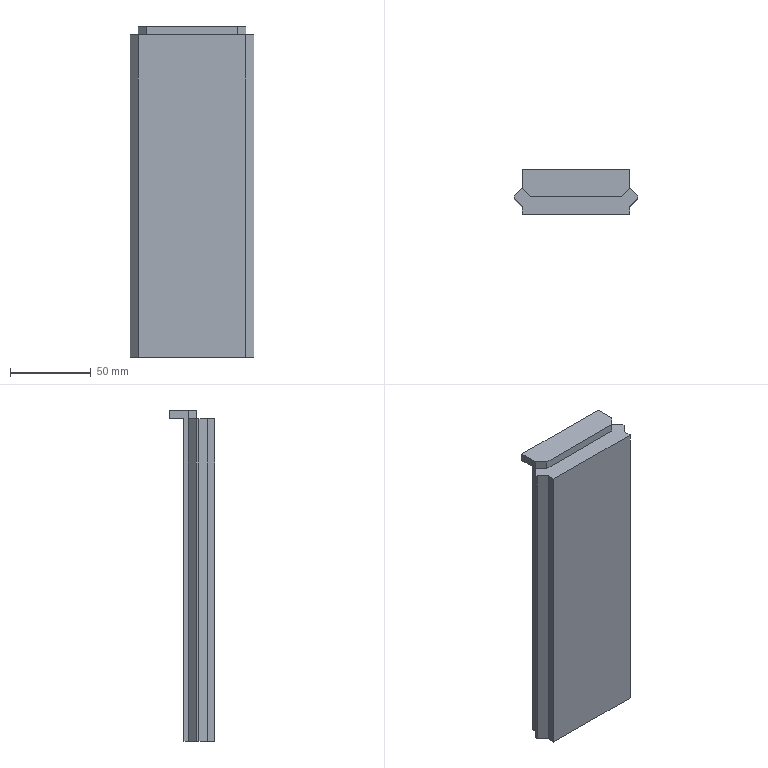Part | SolidWorks | features Chamfer 1, Cut 1, Extrusion 1, ICE 1 | 1 solid | 25 faces | box 77 x 28 x 205 mm | volume 63647 mm3 | plane 25
STEP:
#1=CARTESIAN_POINT('',(-73.,44.353,0.));
#2=VERTEX_POINT('',#1);
#3=CARTESIAN_POINT('',(-73.,44.,0.));
#4=VERTEX_POINT('',#3);
#5=CARTESIAN_POINT('',(-73.,56.,0.));
#6=DIRECTION('',(0.,-1.,0.));
#7=VECTOR('',#6,1000.);
#8=LINE('',#5,#7);
#9=EDGE_CURVE('',#2,#4,#8,.T.);
#10=ORIENTED_EDGE('',*,*,#9,.F.);
#11=CARTESIAN_POINT('',(-78.,39.353,0.));
#12=VERTEX_POINT('',#11);
#13=CARTESIAN_POINT('',(-78.,39.353,0.));
#14=DIRECTION('',(-0.7071,-0.7071,0.));
#15=VECTOR('',#14,1000.);
#16=LINE('',#13,#15);
#17=EDGE_CURVE('',#2,#12,#16,.T.);
#18=ORIENTED_EDGE('',*,*,#17,.T.);
#19=CARTESIAN_POINT('',(-78.,37.657,0.));
#20=VERTEX_POINT('',#19);
#21=CARTESIAN_POINT('',(-78.,37.657,0.));
#22=DIRECTION('',(0.,-1.,0.));
#23=VECTOR('',#22,1000.);
#24=LINE('',#21,#23);
#25=EDGE_CURVE('',#12,#20,#24,.T.);
#26=ORIENTED_EDGE('',*,*,#25,.T.);
#27=CARTESIAN_POINT('',(-73.,32.657,0.));
#28=VERTEX_POINT('',#27);
#29=CARTESIAN_POINT('',(-73.,32.657,0.));
#30=DIRECTION('',(0.7071,-0.7071,0.));
#31=VECTOR('',#30,1000.);
#32=LINE('',#29,#31);
#33=EDGE_CURVE('',#20,#28,#32,.T.);
#34=ORIENTED_EDGE('',*,*,#33,.T.);
#35=CARTESIAN_POINT('',(-73.,28.,0.));
#36=VERTEX_POINT('',#35);
#37=CARTESIAN_POINT('',(-73.,28.,0.));
#38=DIRECTION('',(0.,-1.,0.));
#39=VECTOR('',#38,1000.);
#40=LINE('',#37,#39);
#41=EDGE_CURVE('',#28,#36,#40,.T.);
#42=ORIENTED_EDGE('',*,*,#41,.T.);
#43=CARTESIAN_POINT('',(-6.,28.,0.));
#44=VERTEX_POINT('',#43);
#45=CARTESIAN_POINT('',(-73.,28.,0.));
#46=DIRECTION('',(1.,0.,0.));
#47=VECTOR('',#46,1000.);
#48=LINE('',#45,#47);
#49=EDGE_CURVE('',#36,#44,#48,.T.);
#50=ORIENTED_EDGE('',*,*,#49,.T.);
#51=CARTESIAN_POINT('',(-6.,32.657,0.));
#52=VERTEX_POINT('',#51);
#53=CARTESIAN_POINT('',(-6.,28.,0.));
#54=DIRECTION('',(0.,1.,0.));
#55=VECTOR('',#54,1000.);
#56=LINE('',#53,#55);
#57=EDGE_CURVE('',#44,#52,#56,.T.);
#58=ORIENTED_EDGE('',*,*,#57,.T.);
#59=CARTESIAN_POINT('',(-1.,37.657,0.));
#60=VERTEX_POINT('',#59);
#61=CARTESIAN_POINT('',(-6.,32.657,0.));
#62=DIRECTION('',(0.7071,0.7071,0.));
#63=VECTOR('',#62,1000.);
#64=LINE('',#61,#63);
#65=EDGE_CURVE('',#52,#60,#64,.T.);
#66=ORIENTED_EDGE('',*,*,#65,.T.);
#67=CARTESIAN_POINT('',(-1.,39.353,0.));
#68=VERTEX_POINT('',#67);
#69=CARTESIAN_POINT('',(-1.,37.657,0.));
#70=DIRECTION('',(0.,1.,0.));
#71=VECTOR('',#70,1000.);
#72=LINE('',#69,#71);
#73=EDGE_CURVE('',#60,#68,#72,.T.);
#74=ORIENTED_EDGE('',*,*,#73,.T.);
#75=CARTESIAN_POINT('',(-6.,44.353,0.));
#76=VERTEX_POINT('',#75);
#77=CARTESIAN_POINT('',(-1.,39.353,0.));
#78=DIRECTION('',(-0.7071,0.7071,0.));
#79=VECTOR('',#78,1000.);
#80=LINE('',#77,#79);
#81=EDGE_CURVE('',#68,#76,#80,.T.);
#82=ORIENTED_EDGE('',*,*,#81,.T.);
#83=CARTESIAN_POINT('',(-6.,44.,0.));
#84=VERTEX_POINT('',#83);
#85=CARTESIAN_POINT('',(-6.,56.,0.));
#86=DIRECTION('',(0.,1.,0.));
#87=VECTOR('',#86,1000.);
#88=LINE('',#85,#87);
#89=EDGE_CURVE('',#84,#76,#88,.T.);
#90=ORIENTED_EDGE('',*,*,#89,.F.);
#91=CARTESIAN_POINT('',(-11.,39.,0.));
#92=VERTEX_POINT('',#91);
#93=CARTESIAN_POINT('',(-25.,25.,0.));
#94=DIRECTION('',(-0.7071,-0.7071,0.));
#95=VECTOR('',#94,1000.);
#96=LINE('',#93,#95);
#97=EDGE_CURVE('',#84,#92,#96,.T.);
#98=ORIENTED_EDGE('',*,*,#97,.T.);
#99=CARTESIAN_POINT('',(-68.,39.,0.));
#100=VERTEX_POINT('',#99);
#101=CARTESIAN_POINT('',(-73.,39.,0.));
#102=DIRECTION('',(1.,0.,0.));
#103=VECTOR('',#102,1000.);
#104=LINE('',#101,#103);
#105=EDGE_CURVE('',#100,#92,#104,.T.);
#106=ORIENTED_EDGE('',*,*,#105,.F.);
#107=CARTESIAN_POINT('',(-14.5,-14.5,0.));
#108=DIRECTION('',(-0.7071,0.7071,0.));
#109=VECTOR('',#108,1000.);
#110=LINE('',#107,#109);
#111=EDGE_CURVE('',#100,#4,#110,.T.);
#112=ORIENTED_EDGE('',*,*,#111,.T.);
#113=EDGE_LOOP('',(#10,#18,#26,#34,#42,#50,#58,#66,#74,#82,#90,#98,#106,#112));
#114=FACE_OUTER_BOUND('',#113,.T.);
#115=CARTESIAN_POINT('',(0.,0.,0.));
#116=DIRECTION('',(0.,0.,-1.));
#117=DIRECTION('',(-1.,0.,0.));
#118=AXIS2_PLACEMENT_3D('',#115,#116,#117);
#119=PLANE('',#118);
#120=ADVANCED_FACE('',(#114),#119,.F.);
#121=ORIENTED_EDGE('',*,*,#41,.F.);
#122=CARTESIAN_POINT('',(-73.,32.657,-200.));
#123=VERTEX_POINT('',#122);
#124=CARTESIAN_POINT('',(-73.,32.657,-200.));
#125=DIRECTION('',(0.,0.,1.));
#126=VECTOR('',#125,1000.);
#127=LINE('',#124,#126);
#128=EDGE_CURVE('',#123,#28,#127,.T.);
#129=ORIENTED_EDGE('',*,*,#128,.F.);
#130=CARTESIAN_POINT('',(-73.,28.,-200.));
#131=VERTEX_POINT('',#130);
#132=CARTESIAN_POINT('',(-73.,28.,-200.));
#133=DIRECTION('',(0.,-1.,0.));
#134=VECTOR('',#133,1000.);
#135=LINE('',#132,#134);
#136=EDGE_CURVE('',#123,#131,#135,.T.);
#137=ORIENTED_EDGE('',*,*,#136,.T.);
#138=CARTESIAN_POINT('',(-73.,28.,-200.));
#139=DIRECTION('',(0.,0.,1.));
#140=VECTOR('',#139,1000.);
#141=LINE('',#138,#140);
#142=EDGE_CURVE('',#131,#36,#141,.T.);
#143=ORIENTED_EDGE('',*,*,#142,.T.);
#144=EDGE_LOOP('',(#121,#129,#137,#143));
#145=FACE_OUTER_BOUND('',#144,.T.);
#146=CARTESIAN_POINT('',(-73.,28.,-200.));
#147=DIRECTION('',(-1.,0.,0.));
#148=DIRECTION('',(0.,0.,1.));
#149=AXIS2_PLACEMENT_3D('',#146,#147,#148);
#150=PLANE('',#149);
#151=ADVANCED_FACE('',(#145),#150,.T.);
#152=ORIENTED_EDGE('',*,*,#33,.F.);
#153=CARTESIAN_POINT('',(-78.,37.657,-200.));
#154=VERTEX_POINT('',#153);
#155=CARTESIAN_POINT('',(-78.,37.657,-200.));
#156=DIRECTION('',(0.,0.,1.));
#157=VECTOR('',#156,1000.);
#158=LINE('',#155,#157);
#159=EDGE_CURVE('',#154,#20,#158,.T.);
#160=ORIENTED_EDGE('',*,*,#159,.F.);
#161=CARTESIAN_POINT('',(-73.,32.657,-200.));
#162=DIRECTION('',(0.7071,-0.7071,0.));
#163=VECTOR('',#162,1000.);
#164=LINE('',#161,#163);
#165=EDGE_CURVE('',#154,#123,#164,.T.);
#166=ORIENTED_EDGE('',*,*,#165,.T.);
#167=ORIENTED_EDGE('',*,*,#128,.T.);
#168=EDGE_LOOP('',(#152,#160,#166,#167));
#169=FACE_OUTER_BOUND('',#168,.T.);
#170=CARTESIAN_POINT('',(-73.,32.657,-200.));
#171=DIRECTION('',(-0.7071,-0.7071,0.));
#172=DIRECTION('',(0.7071,-0.7071,0.));
#173=AXIS2_PLACEMENT_3D('',#170,#171,#172);
#174=PLANE('',#173);
#175=ADVANCED_FACE('',(#169),#174,.T.);
#176=ORIENTED_EDGE('',*,*,#25,.F.);
#177=CARTESIAN_POINT('',(-78.,39.353,-200.));
#178=VERTEX_POINT('',#177);
#179=CARTESIAN_POINT('',(-78.,39.353,-200.));
#180=DIRECTION('',(0.,0.,1.));
#181=VECTOR('',#180,1000.);
#182=LINE('',#179,#181);
#183=EDGE_CURVE('',#178,#12,#182,.T.);
#184=ORIENTED_EDGE('',*,*,#183,.F.);
#185=CARTESIAN_POINT('',(-78.,37.657,-200.));
#186=DIRECTION('',(0.,-1.,0.));
#187=VECTOR('',#186,1000.);
#188=LINE('',#185,#187);
#189=EDGE_CURVE('',#178,#154,#188,.T.);
#190=ORIENTED_EDGE('',*,*,#189,.T.);
#191=ORIENTED_EDGE('',*,*,#159,.T.);
#192=EDGE_LOOP('',(#176,#184,#190,#191));
#193=FACE_OUTER_BOUND('',#192,.T.);
#194=CARTESIAN_POINT('',(-78.,37.657,-200.));
#195=DIRECTION('',(-1.,0.,0.));
#196=DIRECTION('',(0.,0.,1.));
#197=AXIS2_PLACEMENT_3D('',#194,#195,#196);
#198=PLANE('',#197);
#199=ADVANCED_FACE('',(#193),#198,.T.);
#200=ORIENTED_EDGE('',*,*,#17,.F.);
#201=CARTESIAN_POINT('',(-73.,44.353,-200.));
#202=VERTEX_POINT('',#201);
#203=CARTESIAN_POINT('',(-73.,44.353,-200.));
#204=DIRECTION('',(0.,0.,1.));
#205=VECTOR('',#204,1000.);
#206=LINE('',#203,#205);
#207=EDGE_CURVE('',#202,#2,#206,.T.);
#208=ORIENTED_EDGE('',*,*,#207,.F.);
#209=CARTESIAN_POINT('',(-78.,39.353,-200.));
#210=DIRECTION('',(-0.7071,-0.7071,0.));
#211=VECTOR('',#210,1000.);
#212=LINE('',#209,#211);
#213=EDGE_CURVE('',#202,#178,#212,.T.);
#214=ORIENTED_EDGE('',*,*,#213,.T.);
#215=ORIENTED_EDGE('',*,*,#183,.T.);
#216=EDGE_LOOP('',(#200,#208,#214,#215));
#217=FACE_OUTER_BOUND('',#216,.T.);
#218=CARTESIAN_POINT('',(-78.,39.353,-200.));
#219=DIRECTION('',(-0.7071,0.7071,0.));
#220=DIRECTION('',(-0.7071,-0.7071,0.));
#221=AXIS2_PLACEMENT_3D('',#218,#219,#220);
#222=PLANE('',#221);
#223=ADVANCED_FACE('',(#217),#222,.T.);
#224=ORIENTED_EDGE('',*,*,#9,.T.);
#225=CARTESIAN_POINT('',(-73.,44.,5.));
#226=VERTEX_POINT('',#225);
#227=CARTESIAN_POINT('',(-73.,44.,5.));
#228=DIRECTION('',(0.,0.,1.));
#229=VECTOR('',#228,1000.);
#230=LINE('',#227,#229);
#231=EDGE_CURVE('',#4,#226,#230,.T.);
#232=ORIENTED_EDGE('',*,*,#231,.T.);
#233=CARTESIAN_POINT('',(-73.,56.,5.));
#234=VERTEX_POINT('',#233);
#235=CARTESIAN_POINT('',(-73.,56.,5.));
#236=DIRECTION('',(0.,-1.,0.));
#237=VECTOR('',#236,1000.);
#238=LINE('',#235,#237);
#239=EDGE_CURVE('',#234,#226,#238,.T.);
#240=ORIENTED_EDGE('',*,*,#239,.F.);
#241=CARTESIAN_POINT('',(-73.,56.,0.));
#242=VERTEX_POINT('',#241);
#243=CARTESIAN_POINT('',(-73.,56.,5.));
#244=DIRECTION('',(0.,0.,-1.));
#245=VECTOR('',#244,1000.);
#246=LINE('',#243,#245);
#247=EDGE_CURVE('',#234,#242,#246,.T.);
#248=ORIENTED_EDGE('',*,*,#247,.T.);
#249=CARTESIAN_POINT('',(-73.,47.,0.));
#250=VERTEX_POINT('',#249);
#251=CARTESIAN_POINT('',(-73.,56.,0.));
#252=DIRECTION('',(0.,-1.,0.));
#253=VECTOR('',#252,1000.);
#254=LINE('',#251,#253);
#255=EDGE_CURVE('',#242,#250,#254,.T.);
#256=ORIENTED_EDGE('',*,*,#255,.T.);
#257=CARTESIAN_POINT('',(-73.,47.,-200.));
#258=VERTEX_POINT('',#257);
#259=CARTESIAN_POINT('',(-73.,47.,-200.));
#260=DIRECTION('',(0.,0.,1.));
#261=VECTOR('',#260,1000.);
#262=LINE('',#259,#261);
#263=EDGE_CURVE('',#258,#250,#262,.T.);
#264=ORIENTED_EDGE('',*,*,#263,.F.);
#265=CARTESIAN_POINT('',(-73.,44.353,-200.));
#266=DIRECTION('',(0.,-1.,0.));
#267=VECTOR('',#266,1000.);
#268=LINE('',#265,#267);
#269=EDGE_CURVE('',#258,#202,#268,.T.);
#270=ORIENTED_EDGE('',*,*,#269,.T.);
#271=ORIENTED_EDGE('',*,*,#207,.T.);
#272=EDGE_LOOP('',(#224,#232,#240,#248,#256,#264,#270,#271));
#273=FACE_OUTER_BOUND('',#272,.T.);
#274=CARTESIAN_POINT('',(-73.,44.353,-200.));
#275=DIRECTION('',(-1.,0.,0.));
#276=DIRECTION('',(0.,0.,1.));
#277=AXIS2_PLACEMENT_3D('',#274,#275,#276);
#278=PLANE('',#277);
#279=ADVANCED_FACE('',(#273),#278,.T.);
#280=CARTESIAN_POINT('',(-71.,47.,-2.));
#281=VERTEX_POINT('',#280);
#282=CARTESIAN_POINT('',(-8.,47.,-2.));
#283=VERTEX_POINT('',#282);
#284=CARTESIAN_POINT('',(-71.,47.,-2.));
#285=DIRECTION('',(1.,0.,0.));
#286=VECTOR('',#285,1000.);
#287=LINE('',#284,#286);
#288=EDGE_CURVE('',#281,#283,#287,.T.);
#289=ORIENTED_EDGE('',*,*,#288,.F.);
#290=CARTESIAN_POINT('',(-71.,47.,-198.));
#291=VERTEX_POINT('',#290);
#292=CARTESIAN_POINT('',(-71.,47.,-198.));
#293=DIRECTION('',(0.,0.,1.));
#294=VECTOR('',#293,1000.);
#295=LINE('',#292,#294);
#296=EDGE_CURVE('',#291,#281,#295,.T.);
#297=ORIENTED_EDGE('',*,*,#296,.F.);
#298=CARTESIAN_POINT('',(-8.,47.,-198.));
#299=VERTEX_POINT('',#298);
#300=CARTESIAN_POINT('',(-8.,47.,-198.));
#301=DIRECTION('',(-1.,0.,0.));
#302=VECTOR('',#301,1000.);
#303=LINE('',#300,#302);
#304=EDGE_CURVE('',#299,#291,#303,.T.);
#305=ORIENTED_EDGE('',*,*,#304,.F.);
#306=CARTESIAN_POINT('',(-8.,47.,-2.));
#307=DIRECTION('',(0.,0.,-1.));
#308=VECTOR('',#307,1000.);
#309=LINE('',#306,#308);
#310=EDGE_CURVE('',#283,#299,#309,.T.);
#311=ORIENTED_EDGE('',*,*,#310,.F.);
#312=EDGE_LOOP('',(#289,#297,#305,#311));
#313=FACE_BOUND('',#312,.T.);
#314=CARTESIAN_POINT('',(-6.,47.,0.));
#315=VERTEX_POINT('',#314);
#316=CARTESIAN_POINT('',(-73.,47.,0.));
#317=DIRECTION('',(-1.,0.,0.));
#318=VECTOR('',#317,1000.);
#319=LINE('',#316,#318);
#320=EDGE_CURVE('',#315,#250,#319,.T.);
#321=ORIENTED_EDGE('',*,*,#320,.F.);
#322=CARTESIAN_POINT('',(-6.,47.,-200.));
#323=VERTEX_POINT('',#322);
#324=CARTESIAN_POINT('',(-6.,47.,-200.));
#325=DIRECTION('',(0.,0.,1.));
#326=VECTOR('',#325,1000.);
#327=LINE('',#324,#326);
#328=EDGE_CURVE('',#323,#315,#327,.T.);
#329=ORIENTED_EDGE('',*,*,#328,.F.);
#330=CARTESIAN_POINT('',(-73.,47.,-200.));
#331=DIRECTION('',(-1.,0.,0.));
#332=VECTOR('',#331,1000.);
#333=LINE('',#330,#332);
#334=EDGE_CURVE('',#323,#258,#333,.T.);
#335=ORIENTED_EDGE('',*,*,#334,.T.);
#336=ORIENTED_EDGE('',*,*,#263,.T.);
#337=EDGE_LOOP('',(#321,#329,#335,#336));
#338=FACE_OUTER_BOUND('',#337,.T.);
#339=CARTESIAN_POINT('',(-73.,47.,-200.));
#340=DIRECTION('',(0.,1.,0.));
#341=DIRECTION('',(-1.,0.,0.));
#342=AXIS2_PLACEMENT_3D('',#339,#340,#341);
#343=PLANE('',#342);
#344=ADVANCED_FACE('',(#313,#338),#343,.T.);
#345=CARTESIAN_POINT('',(-6.,44.,5.));
#346=VERTEX_POINT('',#345);
#347=CARTESIAN_POINT('',(-6.,56.,5.));
#348=VERTEX_POINT('',#347);
#349=CARTESIAN_POINT('',(-6.,56.,5.));
#350=DIRECTION('',(0.,1.,0.));
#351=VECTOR('',#350,1000.);
#352=LINE('',#349,#351);
#353=EDGE_CURVE('',#346,#348,#352,.T.);
#354=ORIENTED_EDGE('',*,*,#353,.F.);
#355=CARTESIAN_POINT('',(-6.,44.,0.));
#356=DIRECTION('',(0.,0.,-1.));
#357=VECTOR('',#356,1000.);
#358=LINE('',#355,#357);
#359=EDGE_CURVE('',#346,#84,#358,.T.);
#360=ORIENTED_EDGE('',*,*,#359,.T.);
#361=ORIENTED_EDGE('',*,*,#89,.T.);
#362=CARTESIAN_POINT('',(-6.,44.353,-200.));
#363=VERTEX_POINT('',#362);
#364=CARTESIAN_POINT('',(-6.,44.353,-200.));
#365=DIRECTION('',(0.,0.,1.));
#366=VECTOR('',#365,1000.);
#367=LINE('',#364,#366);
#368=EDGE_CURVE('',#363,#76,#367,.T.);
#369=ORIENTED_EDGE('',*,*,#368,.F.);
#370=CARTESIAN_POINT('',(-6.,44.353,-200.));
#371=DIRECTION('',(0.,1.,0.));
#372=VECTOR('',#371,1000.);
#373=LINE('',#370,#372);
#374=EDGE_CURVE('',#363,#323,#373,.T.);
#375=ORIENTED_EDGE('',*,*,#374,.T.);
#376=ORIENTED_EDGE('',*,*,#328,.T.);
#377=CARTESIAN_POINT('',(-6.,56.,0.));
#378=VERTEX_POINT('',#377);
#379=CARTESIAN_POINT('',(-6.,56.,0.));
#380=DIRECTION('',(0.,1.,0.));
#381=VECTOR('',#380,1000.);
#382=LINE('',#379,#381);
#383=EDGE_CURVE('',#315,#378,#382,.T.);
#384=ORIENTED_EDGE('',*,*,#383,.T.);
#385=CARTESIAN_POINT('',(-6.,56.,5.));
#386=DIRECTION('',(0.,0.,-1.));
#387=VECTOR('',#386,1000.);
#388=LINE('',#385,#387);
#389=EDGE_CURVE('',#348,#378,#388,.T.);
#390=ORIENTED_EDGE('',*,*,#389,.F.);
#391=EDGE_LOOP('',(#354,#360,#361,#369,#375,#376,#384,#390));
#392=FACE_OUTER_BOUND('',#391,.T.);
#393=CARTESIAN_POINT('',(-6.,44.353,-200.));
#394=DIRECTION('',(1.,0.,0.));
#395=DIRECTION('',(0.,0.,-1.));
#396=AXIS2_PLACEMENT_3D('',#393,#394,#395);
#397=PLANE('',#396);
#398=ADVANCED_FACE('',(#392),#397,.T.);
#399=ORIENTED_EDGE('',*,*,#81,.F.);
#400=CARTESIAN_POINT('',(-1.,39.353,-200.));
#401=VERTEX_POINT('',#400);
#402=CARTESIAN_POINT('',(-1.,39.353,-200.));
#403=DIRECTION('',(0.,0.,1.));
#404=VECTOR('',#403,1000.);
#405=LINE('',#402,#404);
#406=EDGE_CURVE('',#401,#68,#405,.T.);
#407=ORIENTED_EDGE('',*,*,#406,.F.);
#408=CARTESIAN_POINT('',(-1.,39.353,-200.));
#409=DIRECTION('',(-0.7071,0.7071,0.));
#410=VECTOR('',#409,1000.);
#411=LINE('',#408,#410);
#412=EDGE_CURVE('',#401,#363,#411,.T.);
#413=ORIENTED_EDGE('',*,*,#412,.T.);
#414=ORIENTED_EDGE('',*,*,#368,.T.);
#415=EDGE_LOOP('',(#399,#407,#413,#414));
#416=FACE_OUTER_BOUND('',#415,.T.);
#417=CARTESIAN_POINT('',(-1.,39.353,-200.));
#418=DIRECTION('',(0.7071,0.7071,0.));
#419=DIRECTION('',(-0.7071,0.7071,0.));
#420=AXIS2_PLACEMENT_3D('',#417,#418,#419);
#421=PLANE('',#420);
#422=ADVANCED_FACE('',(#416),#421,.T.);
#423=ORIENTED_EDGE('',*,*,#73,.F.);
#424=CARTESIAN_POINT('',(-1.,37.657,-200.));
#425=VERTEX_POINT('',#424);
#426=CARTESIAN_POINT('',(-1.,37.657,-200.));
#427=DIRECTION('',(0.,0.,1.));
#428=VECTOR('',#427,1000.);
#429=LINE('',#426,#428);
#430=EDGE_CURVE('',#425,#60,#429,.T.);
#431=ORIENTED_EDGE('',*,*,#430,.F.);
#432=CARTESIAN_POINT('',(-1.,37.657,-200.));
#433=DIRECTION('',(0.,1.,0.));
#434=VECTOR('',#433,1000.);
#435=LINE('',#432,#434);
#436=EDGE_CURVE('',#425,#401,#435,.T.);
#437=ORIENTED_EDGE('',*,*,#436,.T.);
#438=ORIENTED_EDGE('',*,*,#406,.T.);
#439=EDGE_LOOP('',(#423,#431,#437,#438));
#440=FACE_OUTER_BOUND('',#439,.T.);
#441=CARTESIAN_POINT('',(-1.,37.657,-200.));
#442=DIRECTION('',(1.,0.,0.));
#443=DIRECTION('',(0.,0.,-1.));
#444=AXIS2_PLACEMENT_3D('',#441,#442,#443);
#445=PLANE('',#444);
#446=ADVANCED_FACE('',(#440),#445,.T.);
#447=ORIENTED_EDGE('',*,*,#65,.F.);
#448=CARTESIAN_POINT('',(-6.,32.657,-200.));
#449=VERTEX_POINT('',#448);
#450=CARTESIAN_POINT('',(-6.,32.657,-200.));
#451=DIRECTION('',(0.,0.,1.));
#452=VECTOR('',#451,1000.);
#453=LINE('',#450,#452);
#454=EDGE_CURVE('',#449,#52,#453,.T.);
#455=ORIENTED_EDGE('',*,*,#454,.F.);
#456=CARTESIAN_POINT('',(-6.,32.657,-200.));
#457=DIRECTION('',(0.7071,0.7071,0.));
#458=VECTOR('',#457,1000.);
#459=LINE('',#456,#458);
#460=EDGE_CURVE('',#449,#425,#459,.T.);
#461=ORIENTED_EDGE('',*,*,#460,.T.);
#462=ORIENTED_EDGE('',*,*,#430,.T.);
#463=EDGE_LOOP('',(#447,#455,#461,#462));
#464=FACE_OUTER_BOUND('',#463,.T.);
#465=CARTESIAN_POINT('',(-6.,32.657,-200.));
#466=DIRECTION('',(0.7071,-0.7071,0.));
#467=DIRECTION('',(0.7071,0.7071,0.));
#468=AXIS2_PLACEMENT_3D('',#465,#466,#467);
#469=PLANE('',#468);
#470=ADVANCED_FACE('',(#464),#469,.T.);
#471=ORIENTED_EDGE('',*,*,#57,.F.);
#472=CARTESIAN_POINT('',(-6.,28.,-200.));
#473=VERTEX_POINT('',#472);
#474=CARTESIAN_POINT('',(-6.,28.,-200.));
#475=DIRECTION('',(0.,0.,1.));
#476=VECTOR('',#475,1000.);
#477=LINE('',#474,#476);
#478=EDGE_CURVE('',#473,#44,#477,.T.);
#479=ORIENTED_EDGE('',*,*,#478,.F.);
#480=CARTESIAN_POINT('',(-6.,28.,-200.));
#481=DIRECTION('',(0.,1.,0.));
#482=VECTOR('',#481,1000.);
#483=LINE('',#480,#482);
#484=EDGE_CURVE('',#473,#449,#483,.T.);
#485=ORIENTED_EDGE('',*,*,#484,.T.);
#486=ORIENTED_EDGE('',*,*,#454,.T.);
#487=EDGE_LOOP('',(#471,#479,#485,#486));
#488=FACE_OUTER_BOUND('',#487,.T.);
#489=CARTESIAN_POINT('',(-6.,28.,-200.));
#490=DIRECTION('',(1.,0.,0.));
#491=DIRECTION('',(0.,0.,-1.));
#492=AXIS2_PLACEMENT_3D('',#489,#490,#491);
#493=PLANE('',#492);
#494=ADVANCED_FACE('',(#488),#493,.T.);
#495=ORIENTED_EDGE('',*,*,#49,.F.);
#496=ORIENTED_EDGE('',*,*,#142,.F.);
#497=CARTESIAN_POINT('',(-73.,28.,-200.));
#498=DIRECTION('',(1.,0.,0.));
#499=VECTOR('',#498,1000.);
#500=LINE('',#497,#499);
#501=EDGE_CURVE('',#131,#473,#500,.T.);
#502=ORIENTED_EDGE('',*,*,#501,.T.);
#503=ORIENTED_EDGE('',*,*,#478,.T.);
#504=EDGE_LOOP('',(#495,#496,#502,#503));
#505=FACE_OUTER_BOUND('',#504,.T.);
#506=CARTESIAN_POINT('',(-73.,28.,-200.));
#507=DIRECTION('',(0.,-1.,0.));
#508=DIRECTION('',(1.,0.,0.));
#509=AXIS2_PLACEMENT_3D('',#506,#507,#508);
#510=PLANE('',#509);
#511=ADVANCED_FACE('',(#505),#510,.T.);
#512=ORIENTED_EDGE('',*,*,#136,.F.);
#513=ORIENTED_EDGE('',*,*,#165,.F.);
#514=ORIENTED_EDGE('',*,*,#189,.F.);
#515=ORIENTED_EDGE('',*,*,#213,.F.);
#516=ORIENTED_EDGE('',*,*,#269,.F.);
#517=ORIENTED_EDGE('',*,*,#334,.F.);
#518=ORIENTED_EDGE('',*,*,#374,.F.);
#519=ORIENTED_EDGE('',*,*,#412,.F.);
#520=ORIENTED_EDGE('',*,*,#436,.F.);
#521=ORIENTED_EDGE('',*,*,#460,.F.);
#522=ORIENTED_EDGE('',*,*,#484,.F.);
#523=ORIENTED_EDGE('',*,*,#501,.F.);
#524=EDGE_LOOP('',(#512,#513,#514,#515,#516,#517,#518,#519,#520,#521,#522,#523));
#525=FACE_OUTER_BOUND('',#524,.T.);
#526=CARTESIAN_POINT('',(0.,0.,-200.));
#527=DIRECTION('',(0.,0.,-1.));
#528=DIRECTION('',(-1.,0.,0.));
#529=AXIS2_PLACEMENT_3D('',#526,#527,#528);
#530=PLANE('',#529);
#531=ADVANCED_FACE('',(#525),#530,.T.);
#532=CARTESIAN_POINT('',(-71.,30.,-198.));
#533=VERTEX_POINT('',#532);
#534=CARTESIAN_POINT('',(-71.,30.,-2.));
#535=VERTEX_POINT('',#534);
#536=CARTESIAN_POINT('',(-71.,30.,-198.));
#537=DIRECTION('',(0.,0.,1.));
#538=VECTOR('',#537,1000.);
#539=LINE('',#536,#538);
#540=EDGE_CURVE('',#533,#535,#539,.T.);
#541=ORIENTED_EDGE('',*,*,#540,.T.);
#542=CARTESIAN_POINT('',(-8.,30.,-2.));
#543=VERTEX_POINT('',#542);
#544=CARTESIAN_POINT('',(-71.,30.,-2.));
#545=DIRECTION('',(1.,0.,0.));
#546=VECTOR('',#545,1000.);
#547=LINE('',#544,#546);
#548=EDGE_CURVE('',#535,#543,#547,.T.);
#549=ORIENTED_EDGE('',*,*,#548,.T.);
#550=CARTESIAN_POINT('',(-8.,30.,-198.));
#551=VERTEX_POINT('',#550);
#552=CARTESIAN_POINT('',(-8.,30.,-2.));
#553=DIRECTION('',(0.,0.,-1.));
#554=VECTOR('',#553,1000.);
#555=LINE('',#552,#554);
#556=EDGE_CURVE('',#543,#551,#555,.T.);
#557=ORIENTED_EDGE('',*,*,#556,.T.);
#558=CARTESIAN_POINT('',(-8.,30.,-198.));
#559=DIRECTION('',(-1.,0.,0.));
#560=VECTOR('',#559,1000.);
#561=LINE('',#558,#560);
#562=EDGE_CURVE('',#551,#533,#561,.T.);
#563=ORIENTED_EDGE('',*,*,#562,.T.);
#564=EDGE_LOOP('',(#541,#549,#557,#563));
#565=FACE_OUTER_BOUND('',#564,.T.);
#566=CARTESIAN_POINT('',(-73.,30.,-200.));
#567=DIRECTION('',(0.,-1.,0.));
#568=DIRECTION('',(1.,0.,0.));
#569=AXIS2_PLACEMENT_3D('',#566,#567,#568);
#570=PLANE('',#569);
#571=ADVANCED_FACE('',(#565),#570,.F.);
#572=CARTESIAN_POINT('',(-71.,-177.876,-2.));
#573=DIRECTION('',(0.,1.,0.));
#574=VECTOR('',#573,1000.);
#575=LINE('',#572,#574);
#576=EDGE_CURVE('',#535,#281,#575,.T.);
#577=ORIENTED_EDGE('',*,*,#576,.T.);
#578=ORIENTED_EDGE('',*,*,#288,.T.);
#579=CARTESIAN_POINT('',(-8.,-177.876,-2.));
#580=DIRECTION('',(0.,1.,0.));
#581=VECTOR('',#580,1000.);
#582=LINE('',#579,#581);
#583=EDGE_CURVE('',#543,#283,#582,.T.);
#584=ORIENTED_EDGE('',*,*,#583,.F.);
#585=ORIENTED_EDGE('',*,*,#548,.F.);
#586=EDGE_LOOP('',(#577,#578,#584,#585));
#587=FACE_OUTER_BOUND('',#586,.T.);
#588=CARTESIAN_POINT('',(-71.,-177.876,-2.));
#589=DIRECTION('',(0.,0.,1.));
#590=DIRECTION('',(1.,0.,0.));
#591=AXIS2_PLACEMENT_3D('',#588,#589,#590);
#592=PLANE('',#591);
#593=ADVANCED_FACE('',(#587),#592,.F.);
#594=ORIENTED_EDGE('',*,*,#583,.T.);
#595=ORIENTED_EDGE('',*,*,#310,.T.);
#596=CARTESIAN_POINT('',(-8.,-177.876,-198.));
#597=DIRECTION('',(0.,1.,0.));
#598=VECTOR('',#597,1000.);
#599=LINE('',#596,#598);
#600=EDGE_CURVE('',#551,#299,#599,.T.);
#601=ORIENTED_EDGE('',*,*,#600,.F.);
#602=ORIENTED_EDGE('',*,*,#556,.F.);
#603=EDGE_LOOP('',(#594,#595,#601,#602));
#604=FACE_OUTER_BOUND('',#603,.T.);
#605=CARTESIAN_POINT('',(-8.,-177.876,-2.));
#606=DIRECTION('',(1.,0.,0.));
#607=DIRECTION('',(0.,1.,0.));
#608=AXIS2_PLACEMENT_3D('',#605,#606,#607);
#609=PLANE('',#608);
#610=ADVANCED_FACE('',(#604),#609,.F.);
#611=ORIENTED_EDGE('',*,*,#600,.T.);
#612=ORIENTED_EDGE('',*,*,#304,.T.);
#613=CARTESIAN_POINT('',(-71.,-177.876,-198.));
#614=DIRECTION('',(0.,1.,0.));
#615=VECTOR('',#614,1000.);
#616=LINE('',#613,#615);
#617=EDGE_CURVE('',#533,#291,#616,.T.);
#618=ORIENTED_EDGE('',*,*,#617,.F.);
#619=ORIENTED_EDGE('',*,*,#562,.F.);
#620=EDGE_LOOP('',(#611,#612,#618,#619));
#621=FACE_OUTER_BOUND('',#620,.T.);
#622=CARTESIAN_POINT('',(-8.,-177.876,-198.));
#623=DIRECTION('',(0.,0.,-1.));
#624=DIRECTION('',(-1.,0.,0.));
#625=AXIS2_PLACEMENT_3D('',#622,#623,#624);
#626=PLANE('',#625);
#627=ADVANCED_FACE('',(#621),#626,.F.);
#628=ORIENTED_EDGE('',*,*,#617,.T.);
#629=ORIENTED_EDGE('',*,*,#296,.T.);
#630=ORIENTED_EDGE('',*,*,#576,.F.);
#631=ORIENTED_EDGE('',*,*,#540,.F.);
#632=EDGE_LOOP('',(#628,#629,#630,#631));
#633=FACE_OUTER_BOUND('',#632,.T.);
#634=CARTESIAN_POINT('',(-71.,-177.876,-198.));
#635=DIRECTION('',(-1.,0.,0.));
#636=DIRECTION('',(0.,-1.,0.));
#637=AXIS2_PLACEMENT_3D('',#634,#635,#636);
#638=PLANE('',#637);
#639=ADVANCED_FACE('',(#633),#638,.F.);
#640=ORIENTED_EDGE('',*,*,#383,.F.);
#641=ORIENTED_EDGE('',*,*,#320,.T.);
#642=ORIENTED_EDGE('',*,*,#255,.F.);
#643=CARTESIAN_POINT('',(-73.,56.,0.));
#644=DIRECTION('',(-1.,0.,0.));
#645=VECTOR('',#644,1000.);
#646=LINE('',#643,#645);
#647=EDGE_CURVE('',#378,#242,#646,.T.);
#648=ORIENTED_EDGE('',*,*,#647,.F.);
#649=EDGE_LOOP('',(#640,#641,#642,#648));
#650=FACE_OUTER_BOUND('',#649,.T.);
#651=CARTESIAN_POINT('',(0.,0.,0.));
#652=DIRECTION('',(0.,0.,1.));
#653=DIRECTION('',(1.,0.,0.));
#654=AXIS2_PLACEMENT_3D('',#651,#652,#653);
#655=PLANE('',#654);
#656=ADVANCED_FACE('',(#650),#655,.F.);
#657=CARTESIAN_POINT('',(-68.,39.,5.));
#658=VERTEX_POINT('',#657);
#659=CARTESIAN_POINT('',(-11.,39.,5.));
#660=VERTEX_POINT('',#659);
#661=CARTESIAN_POINT('',(-73.,39.,5.));
#662=DIRECTION('',(1.,0.,0.));
#663=VECTOR('',#662,1000.);
#664=LINE('',#661,#663);
#665=EDGE_CURVE('',#658,#660,#664,.T.);
#666=ORIENTED_EDGE('',*,*,#665,.F.);
#667=CARTESIAN_POINT('',(-68.,39.,0.));
#668=DIRECTION('',(0.,0.,-1.));
#669=VECTOR('',#668,1000.);
#670=LINE('',#667,#669);
#671=EDGE_CURVE('',#658,#100,#670,.T.);
#672=ORIENTED_EDGE('',*,*,#671,.T.);
#673=ORIENTED_EDGE('',*,*,#105,.T.);
#674=CARTESIAN_POINT('',(-11.,39.,5.));
#675=DIRECTION('',(0.,0.,1.));
#676=VECTOR('',#675,1000.);
#677=LINE('',#674,#676);
#678=EDGE_CURVE('',#92,#660,#677,.T.);
#679=ORIENTED_EDGE('',*,*,#678,.T.);
#680=EDGE_LOOP('',(#666,#672,#673,#679));
#681=FACE_OUTER_BOUND('',#680,.T.);
#682=CARTESIAN_POINT('',(-73.,39.,5.));
#683=DIRECTION('',(0.,1.,0.));
#684=DIRECTION('',(0.,0.,1.));
#685=AXIS2_PLACEMENT_3D('',#682,#683,#684);
#686=PLANE('',#685);
#687=ADVANCED_FACE('',(#681),#686,.F.);
#688=ORIENTED_EDGE('',*,*,#647,.T.);
#689=ORIENTED_EDGE('',*,*,#247,.F.);
#690=CARTESIAN_POINT('',(-73.,56.,5.));
#691=DIRECTION('',(-1.,0.,0.));
#692=VECTOR('',#691,1000.);
#693=LINE('',#690,#692);
#694=EDGE_CURVE('',#348,#234,#693,.T.);
#695=ORIENTED_EDGE('',*,*,#694,.F.);
#696=ORIENTED_EDGE('',*,*,#389,.T.);
#697=EDGE_LOOP('',(#688,#689,#695,#696));
#698=FACE_OUTER_BOUND('',#697,.T.);
#699=CARTESIAN_POINT('',(-73.,56.,5.));
#700=DIRECTION('',(0.,-1.,0.));
#701=DIRECTION('',(0.,0.,-1.));
#702=AXIS2_PLACEMENT_3D('',#699,#700,#701);
#703=PLANE('',#702);
#704=ADVANCED_FACE('',(#698),#703,.F.);
#705=ORIENTED_EDGE('',*,*,#239,.T.);
#706=CARTESIAN_POINT('',(-14.5,-14.5,5.));
#707=DIRECTION('',(0.7071,-0.7071,0.));
#708=VECTOR('',#707,1000.);
#709=LINE('',#706,#708);
#710=EDGE_CURVE('',#226,#658,#709,.T.);
#711=ORIENTED_EDGE('',*,*,#710,.T.);
#712=ORIENTED_EDGE('',*,*,#665,.T.);
#713=CARTESIAN_POINT('',(-25.,25.,5.));
#714=DIRECTION('',(0.7071,0.7071,0.));
#715=VECTOR('',#714,1000.);
#716=LINE('',#713,#715);
#717=EDGE_CURVE('',#660,#346,#716,.T.);
#718=ORIENTED_EDGE('',*,*,#717,.T.);
#719=ORIENTED_EDGE('',*,*,#353,.T.);
#720=ORIENTED_EDGE('',*,*,#694,.T.);
#721=EDGE_LOOP('',(#705,#711,#712,#718,#719,#720));
#722=FACE_OUTER_BOUND('',#721,.T.);
#723=CARTESIAN_POINT('',(0.,0.,5.));
#724=DIRECTION('',(0.,0.,1.));
#725=DIRECTION('',(1.,0.,0.));
#726=AXIS2_PLACEMENT_3D('',#723,#724,#725);
#727=PLANE('',#726);
#728=ADVANCED_FACE('',(#722),#727,.T.);
#729=ORIENTED_EDGE('',*,*,#710,.F.);
#730=ORIENTED_EDGE('',*,*,#231,.F.);
#731=ORIENTED_EDGE('',*,*,#111,.F.);
#732=ORIENTED_EDGE('',*,*,#671,.F.);
#733=EDGE_LOOP('',(#729,#730,#731,#732));
#734=FACE_OUTER_BOUND('',#733,.T.);
#735=CARTESIAN_POINT('',(-68.,39.,5.));
#736=DIRECTION('',(-0.7071,-0.7071,0.));
#737=DIRECTION('',(0.,0.,1.));
#738=AXIS2_PLACEMENT_3D('',#735,#736,#737);
#739=PLANE('',#738);
#740=ADVANCED_FACE('',(#734),#739,.T.);
#741=ORIENTED_EDGE('',*,*,#717,.F.);
#742=ORIENTED_EDGE('',*,*,#678,.F.);
#743=ORIENTED_EDGE('',*,*,#97,.F.);
#744=ORIENTED_EDGE('',*,*,#359,.F.);
#745=EDGE_LOOP('',(#741,#742,#743,#744));
#746=FACE_OUTER_BOUND('',#745,.T.);
#747=CARTESIAN_POINT('',(-6.,44.,-200.));
#748=DIRECTION('',(0.7071,-0.7071,0.));
#749=DIRECTION('',(0.,0.,1.));
#750=AXIS2_PLACEMENT_3D('',#747,#748,#749);
#751=PLANE('',#750);
#752=ADVANCED_FACE('',(#746),#751,.T.);
#753=CLOSED_SHELL('',(#120,#151,#175,#199,#223,#279,#344,#398,#422,#446,#470,#494,#511,#531,#571,#593,#610,#627,#639,#656,#687,#704,#728,#740,#752));
#754=MANIFOLD_SOLID_BREP('',#753);
#755=CARTESIAN_POINT('',(0.,0.,0.));
#756=DIRECTION('',(0.,0.,1.));
#757=DIRECTION('',(1.,0.,0.));
#758=AXIS2_PLACEMENT_3D('',#755,#756,#757);
#759=(LENGTH_UNIT()NAMED_UNIT(*)SI_UNIT(.MILLI.,.METRE.));
#760=UNCERTAINTY_MEASURE_WITH_UNIT(LENGTH_MEASURE(0.00001),#759,'','');
#761=(NAMED_UNIT(*)PLANE_ANGLE_UNIT()SI_UNIT($,.RADIAN.));
#762=(NAMED_UNIT(*)SI_UNIT($,.STERADIAN.)SOLID_ANGLE_UNIT());
#763=(GEOMETRIC_REPRESENTATION_CONTEXT(3)GLOBAL_UNCERTAINTY_ASSIGNED_CONTEXT((#760))GLOBAL_UNIT_ASSIGNED_CONTEXT((#759,#761,#762))REPRESENTATION_CONTEXT('',''));
#764=ADVANCED_BREP_SHAPE_REPRESENTATION('',(#754,#758),#763);